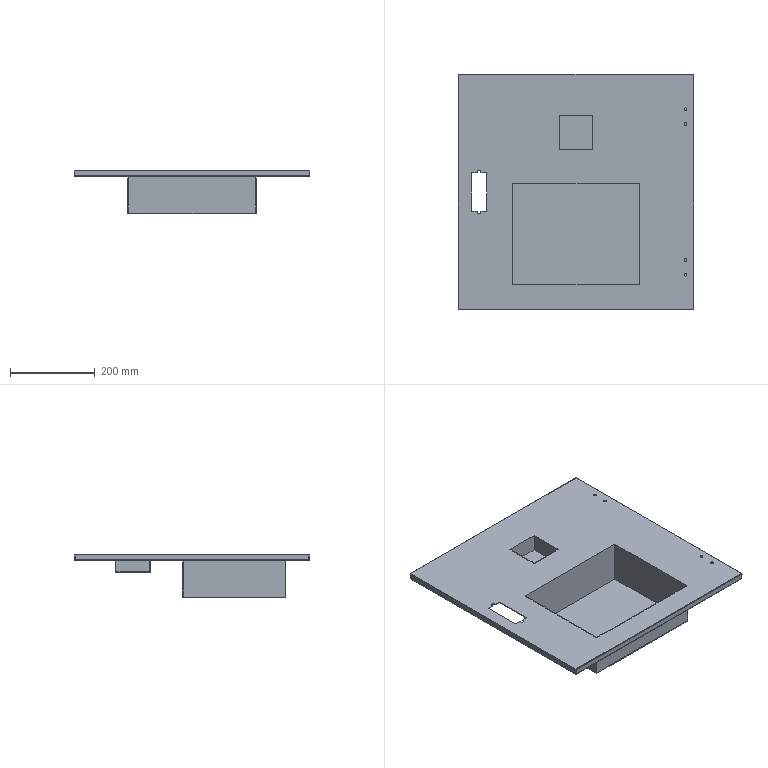Part | STEP file | Right door panel sheet metal_PN_0005 | 1 solid | 110 faces | box 558 x 557 x 103 mm | volume 763625 mm3 | plane 68 | cylinder 26 | spline 16 | commonest cylinder face diameters 0.2 x8 3.2 x8 6.5 x8 8 x2